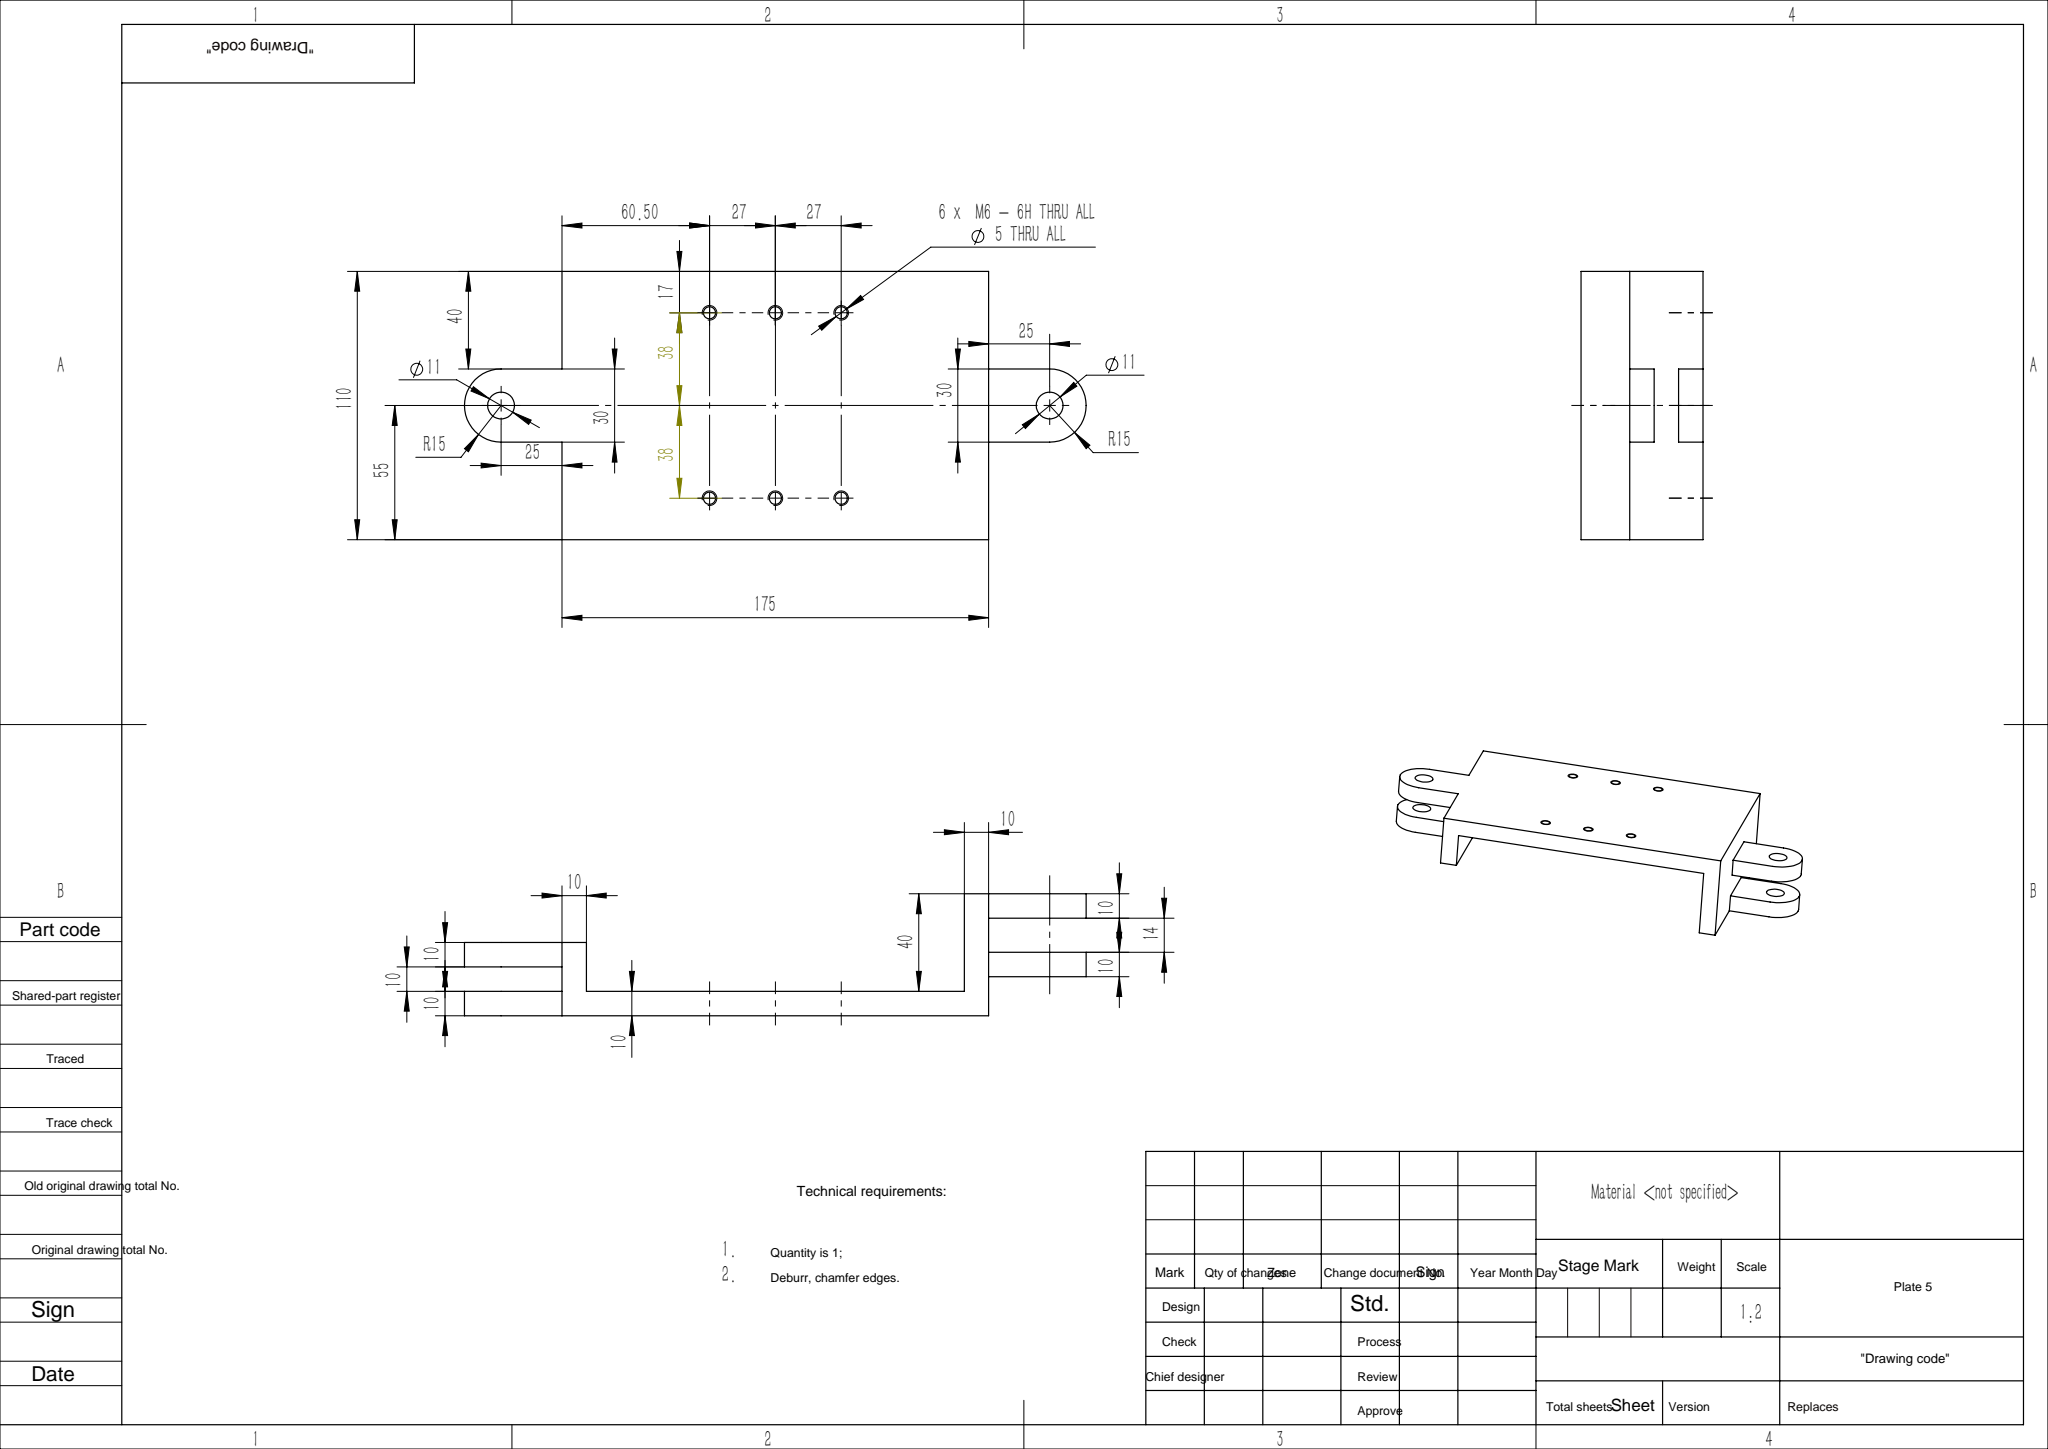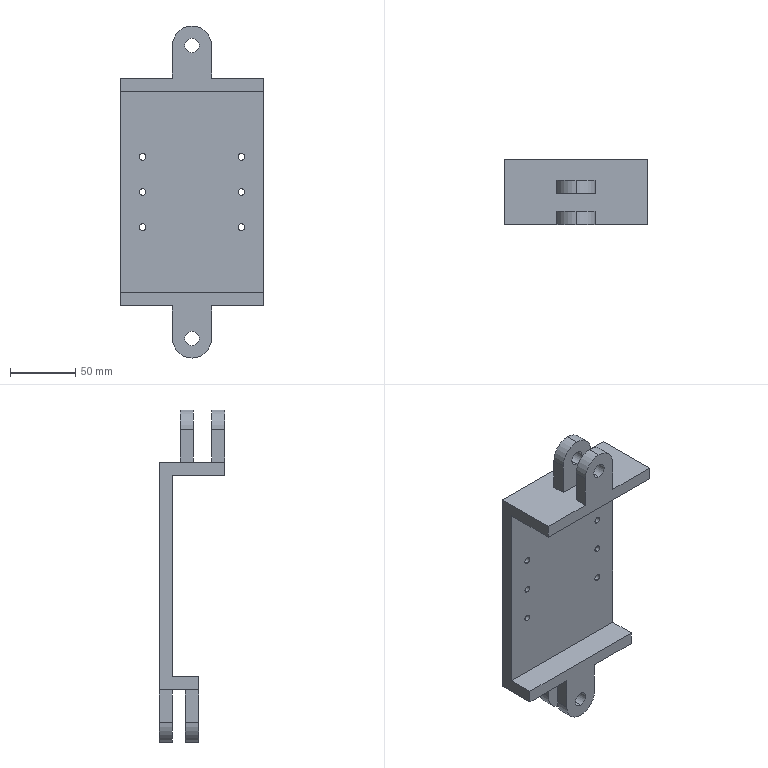Part | SolidWorks | features ICE 6, Fillet 2, LPattern 2, Extrusion 1, HoleWzd 1 | 1 solid | 51 faces | box 110 x 50 x 255 mm | volume 297658 mm3 | cylinder 28 | plane 23 | commonest cylinder face diameters 5 x12 11 x8 30 x8